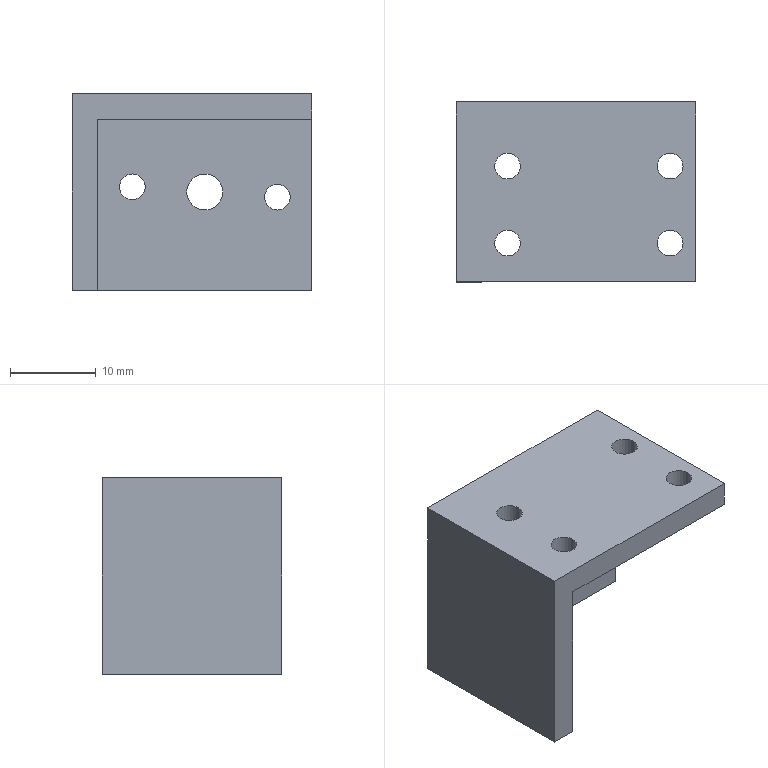Part | SolidWorks | features ICE 2, Extrusion 1 | 1 solid | 23 faces | box 28 x 21 x 23 mm | volume 4355 mm3 | cylinder 14 | plane 9 | commonest cylinder face diameters 3 x12 4.2 x2
STEP:
#1=CARTESIAN_POINT('',(8.478,12.,-10.616));
#2=VERTEX_POINT('',#1);
#3=CARTESIAN_POINT('',(8.478,12.,-7.616));
#4=VERTEX_POINT('',#3);
#5=CARTESIAN_POINT('',(8.478,12.,-9.116));
#6=DIRECTION('',(0.,1.,0.));
#7=DIRECTION('',(0.,0.,1.));
#8=AXIS2_PLACEMENT_3D('',#5,#6,#7);
#9=CIRCLE('',#8,1.5);
#10=EDGE_CURVE('',#2,#4,#9,.T.);
#11=ORIENTED_EDGE('',*,*,#10,.T.);
#12=CARTESIAN_POINT('',(8.478,9.,-7.616));
#13=VERTEX_POINT('',#12);
#14=CARTESIAN_POINT('',(8.478,12.,-7.616));
#15=DIRECTION('',(0.,-1.,0.));
#16=VECTOR('',#15,1000.);
#17=LINE('',#14,#16);
#18=EDGE_CURVE('',#4,#13,#17,.T.);
#19=ORIENTED_EDGE('',*,*,#18,.T.);
#20=CARTESIAN_POINT('',(8.478,9.,-10.616));
#21=VERTEX_POINT('',#20);
#22=CARTESIAN_POINT('',(8.478,9.,-9.116));
#23=DIRECTION('',(0.,1.,0.));
#24=DIRECTION('',(0.,0.,1.));
#25=AXIS2_PLACEMENT_3D('',#22,#23,#24);
#26=CIRCLE('',#25,1.5);
#27=EDGE_CURVE('',#21,#13,#26,.T.);
#28=ORIENTED_EDGE('',*,*,#27,.F.);
#29=CARTESIAN_POINT('',(8.478,12.,-10.616));
#30=DIRECTION('',(0.,-1.,0.));
#31=VECTOR('',#30,1000.);
#32=LINE('',#29,#31);
#33=EDGE_CURVE('',#2,#21,#32,.T.);
#34=ORIENTED_EDGE('',*,*,#33,.F.);
#35=EDGE_LOOP('',(#11,#19,#28,#34));
#36=FACE_OUTER_BOUND('',#35,.T.);
#37=CARTESIAN_POINT('',(8.478,12.,-9.116));
#38=DIRECTION('',(0.,-1.,0.));
#39=DIRECTION('',(0.,0.,-1.));
#40=AXIS2_PLACEMENT_3D('',#37,#38,#39);
#41=CYLINDRICAL_SURFACE('',#40,1.5);
#42=ADVANCED_FACE('',(#36),#41,.F.);
#43=CARTESIAN_POINT('',(-8.478,12.,-9.384));
#44=VERTEX_POINT('',#43);
#45=CARTESIAN_POINT('',(-8.478,12.,-6.384));
#46=VERTEX_POINT('',#45);
#47=CARTESIAN_POINT('',(-8.478,12.,-7.884));
#48=DIRECTION('',(0.,1.,0.));
#49=DIRECTION('',(0.,0.,1.));
#50=AXIS2_PLACEMENT_3D('',#47,#48,#49);
#51=CIRCLE('',#50,1.5);
#52=EDGE_CURVE('',#44,#46,#51,.T.);
#53=ORIENTED_EDGE('',*,*,#52,.T.);
#54=CARTESIAN_POINT('',(-8.478,9.,-6.384));
#55=VERTEX_POINT('',#54);
#56=CARTESIAN_POINT('',(-8.478,12.,-6.384));
#57=DIRECTION('',(0.,-1.,0.));
#58=VECTOR('',#57,1000.);
#59=LINE('',#56,#58);
#60=EDGE_CURVE('',#46,#55,#59,.T.);
#61=ORIENTED_EDGE('',*,*,#60,.T.);
#62=CARTESIAN_POINT('',(-8.478,9.,-9.384));
#63=VERTEX_POINT('',#62);
#64=CARTESIAN_POINT('',(-8.478,9.,-7.884));
#65=DIRECTION('',(0.,1.,0.));
#66=DIRECTION('',(0.,0.,1.));
#67=AXIS2_PLACEMENT_3D('',#64,#65,#66);
#68=CIRCLE('',#67,1.5);
#69=EDGE_CURVE('',#63,#55,#68,.T.);
#70=ORIENTED_EDGE('',*,*,#69,.F.);
#71=CARTESIAN_POINT('',(-8.478,12.,-9.384));
#72=DIRECTION('',(0.,-1.,0.));
#73=VECTOR('',#72,1000.);
#74=LINE('',#71,#73);
#75=EDGE_CURVE('',#44,#63,#74,.T.);
#76=ORIENTED_EDGE('',*,*,#75,.F.);
#77=EDGE_LOOP('',(#53,#61,#70,#76));
#78=FACE_OUTER_BOUND('',#77,.T.);
#79=CARTESIAN_POINT('',(-8.478,12.,-7.884));
#80=DIRECTION('',(0.,-1.,0.));
#81=DIRECTION('',(0.,0.,-1.));
#82=AXIS2_PLACEMENT_3D('',#79,#80,#81);
#83=CYLINDRICAL_SURFACE('',#82,1.5);
#84=ADVANCED_FACE('',(#78),#83,.F.);
#85=CARTESIAN_POINT('',(0.,12.,-10.6));
#86=VERTEX_POINT('',#85);
#87=CARTESIAN_POINT('',(0.,12.,-6.4));
#88=VERTEX_POINT('',#87);
#89=CARTESIAN_POINT('',(0.,12.,-8.5));
#90=DIRECTION('',(0.,1.,0.));
#91=DIRECTION('',(0.,0.,1.));
#92=AXIS2_PLACEMENT_3D('',#89,#90,#91);
#93=CIRCLE('',#92,2.1);
#94=EDGE_CURVE('',#86,#88,#93,.T.);
#95=ORIENTED_EDGE('',*,*,#94,.T.);
#96=CARTESIAN_POINT('',(0.,9.,-6.4));
#97=VERTEX_POINT('',#96);
#98=CARTESIAN_POINT('',(0.,12.,-6.4));
#99=DIRECTION('',(0.,-1.,0.));
#100=VECTOR('',#99,1000.);
#101=LINE('',#98,#100);
#102=EDGE_CURVE('',#88,#97,#101,.T.);
#103=ORIENTED_EDGE('',*,*,#102,.T.);
#104=CARTESIAN_POINT('',(0.,9.,-10.6));
#105=VERTEX_POINT('',#104);
#106=CARTESIAN_POINT('',(0.,9.,-8.5));
#107=DIRECTION('',(0.,1.,0.));
#108=DIRECTION('',(0.,0.,1.));
#109=AXIS2_PLACEMENT_3D('',#106,#107,#108);
#110=CIRCLE('',#109,2.1);
#111=EDGE_CURVE('',#105,#97,#110,.T.);
#112=ORIENTED_EDGE('',*,*,#111,.F.);
#113=CARTESIAN_POINT('',(0.,12.,-10.6));
#114=DIRECTION('',(0.,-1.,0.));
#115=VECTOR('',#114,1000.);
#116=LINE('',#113,#115);
#117=EDGE_CURVE('',#86,#105,#116,.T.);
#118=ORIENTED_EDGE('',*,*,#117,.F.);
#119=EDGE_LOOP('',(#95,#103,#112,#118));
#120=FACE_OUTER_BOUND('',#119,.T.);
#121=CARTESIAN_POINT('',(0.,12.,-8.5));
#122=DIRECTION('',(0.,-1.,0.));
#123=DIRECTION('',(0.,0.,-1.));
#124=AXIS2_PLACEMENT_3D('',#121,#122,#123);
#125=CYLINDRICAL_SURFACE('',#124,2.1);
#126=ADVANCED_FACE('',(#120),#125,.F.);
#127=CARTESIAN_POINT('',(-11.,-4.5,3.));
#128=VERTEX_POINT('',#127);
#129=CARTESIAN_POINT('',(-8.,-4.5,3.));
#130=VERTEX_POINT('',#129);
#131=CARTESIAN_POINT('',(-9.5,-4.5,3.));
#132=DIRECTION('',(0.,0.,1.));
#133=DIRECTION('',(1.,0.,0.));
#134=AXIS2_PLACEMENT_3D('',#131,#132,#133);
#135=CIRCLE('',#134,1.5);
#136=EDGE_CURVE('',#128,#130,#135,.T.);
#137=ORIENTED_EDGE('',*,*,#136,.T.);
#138=CARTESIAN_POINT('',(-8.,-4.5,0.));
#139=VERTEX_POINT('',#138);
#140=CARTESIAN_POINT('',(-8.,-4.5,3.));
#141=DIRECTION('',(0.,0.,-1.));
#142=VECTOR('',#141,1000.);
#143=LINE('',#140,#142);
#144=EDGE_CURVE('',#130,#139,#143,.T.);
#145=ORIENTED_EDGE('',*,*,#144,.T.);
#146=CARTESIAN_POINT('',(-11.,-4.5,0.));
#147=VERTEX_POINT('',#146);
#148=CARTESIAN_POINT('',(-9.5,-4.5,0.));
#149=DIRECTION('',(0.,0.,1.));
#150=DIRECTION('',(1.,0.,0.));
#151=AXIS2_PLACEMENT_3D('',#148,#149,#150);
#152=CIRCLE('',#151,1.5);
#153=EDGE_CURVE('',#147,#139,#152,.T.);
#154=ORIENTED_EDGE('',*,*,#153,.F.);
#155=CARTESIAN_POINT('',(-11.,-4.5,3.));
#156=DIRECTION('',(0.,0.,-1.));
#157=VECTOR('',#156,1000.);
#158=LINE('',#155,#157);
#159=EDGE_CURVE('',#128,#147,#158,.T.);
#160=ORIENTED_EDGE('',*,*,#159,.F.);
#161=EDGE_LOOP('',(#137,#145,#154,#160));
#162=FACE_OUTER_BOUND('',#161,.T.);
#163=CARTESIAN_POINT('',(-9.5,-4.5,3.));
#164=DIRECTION('',(0.,0.,-1.));
#165=DIRECTION('',(-1.,0.,0.));
#166=AXIS2_PLACEMENT_3D('',#163,#164,#165);
#167=CYLINDRICAL_SURFACE('',#166,1.5);
#168=ADVANCED_FACE('',(#162),#167,.F.);
#169=CARTESIAN_POINT('',(8.,-4.5,3.));
#170=VERTEX_POINT('',#169);
#171=CARTESIAN_POINT('',(11.,-4.5,3.));
#172=VERTEX_POINT('',#171);
#173=CARTESIAN_POINT('',(9.5,-4.5,3.));
#174=DIRECTION('',(0.,0.,1.));
#175=DIRECTION('',(1.,0.,0.));
#176=AXIS2_PLACEMENT_3D('',#173,#174,#175);
#177=CIRCLE('',#176,1.5);
#178=EDGE_CURVE('',#170,#172,#177,.T.);
#179=ORIENTED_EDGE('',*,*,#178,.T.);
#180=CARTESIAN_POINT('',(11.,-4.5,0.));
#181=VERTEX_POINT('',#180);
#182=CARTESIAN_POINT('',(11.,-4.5,3.));
#183=DIRECTION('',(0.,0.,-1.));
#184=VECTOR('',#183,1000.);
#185=LINE('',#182,#184);
#186=EDGE_CURVE('',#172,#181,#185,.T.);
#187=ORIENTED_EDGE('',*,*,#186,.T.);
#188=CARTESIAN_POINT('',(8.,-4.5,0.));
#189=VERTEX_POINT('',#188);
#190=CARTESIAN_POINT('',(9.5,-4.5,0.));
#191=DIRECTION('',(0.,0.,1.));
#192=DIRECTION('',(1.,0.,0.));
#193=AXIS2_PLACEMENT_3D('',#190,#191,#192);
#194=CIRCLE('',#193,1.5);
#195=EDGE_CURVE('',#189,#181,#194,.T.);
#196=ORIENTED_EDGE('',*,*,#195,.F.);
#197=CARTESIAN_POINT('',(8.,-4.5,3.));
#198=DIRECTION('',(0.,0.,-1.));
#199=VECTOR('',#198,1000.);
#200=LINE('',#197,#199);
#201=EDGE_CURVE('',#170,#189,#200,.T.);
#202=ORIENTED_EDGE('',*,*,#201,.F.);
#203=EDGE_LOOP('',(#179,#187,#196,#202));
#204=FACE_OUTER_BOUND('',#203,.T.);
#205=CARTESIAN_POINT('',(9.5,-4.5,3.));
#206=DIRECTION('',(0.,0.,-1.));
#207=DIRECTION('',(-1.,0.,0.));
#208=AXIS2_PLACEMENT_3D('',#205,#206,#207);
#209=CYLINDRICAL_SURFACE('',#208,1.5);
#210=ADVANCED_FACE('',(#204),#209,.F.);
#211=CARTESIAN_POINT('',(8.,4.5,3.));
#212=VERTEX_POINT('',#211);
#213=CARTESIAN_POINT('',(11.,4.5,3.));
#214=VERTEX_POINT('',#213);
#215=CARTESIAN_POINT('',(9.5,4.5,3.));
#216=DIRECTION('',(0.,0.,1.));
#217=DIRECTION('',(1.,0.,0.));
#218=AXIS2_PLACEMENT_3D('',#215,#216,#217);
#219=CIRCLE('',#218,1.5);
#220=EDGE_CURVE('',#212,#214,#219,.T.);
#221=ORIENTED_EDGE('',*,*,#220,.T.);
#222=CARTESIAN_POINT('',(11.,4.5,0.));
#223=VERTEX_POINT('',#222);
#224=CARTESIAN_POINT('',(11.,4.5,3.));
#225=DIRECTION('',(0.,0.,-1.));
#226=VECTOR('',#225,1000.);
#227=LINE('',#224,#226);
#228=EDGE_CURVE('',#214,#223,#227,.T.);
#229=ORIENTED_EDGE('',*,*,#228,.T.);
#230=CARTESIAN_POINT('',(8.,4.5,0.));
#231=VERTEX_POINT('',#230);
#232=CARTESIAN_POINT('',(9.5,4.5,0.));
#233=DIRECTION('',(0.,0.,1.));
#234=DIRECTION('',(1.,0.,0.));
#235=AXIS2_PLACEMENT_3D('',#232,#233,#234);
#236=CIRCLE('',#235,1.5);
#237=EDGE_CURVE('',#231,#223,#236,.T.);
#238=ORIENTED_EDGE('',*,*,#237,.F.);
#239=CARTESIAN_POINT('',(8.,4.5,3.));
#240=DIRECTION('',(0.,0.,-1.));
#241=VECTOR('',#240,1000.);
#242=LINE('',#239,#241);
#243=EDGE_CURVE('',#212,#231,#242,.T.);
#244=ORIENTED_EDGE('',*,*,#243,.F.);
#245=EDGE_LOOP('',(#221,#229,#238,#244));
#246=FACE_OUTER_BOUND('',#245,.T.);
#247=CARTESIAN_POINT('',(9.5,4.5,3.));
#248=DIRECTION('',(0.,0.,-1.));
#249=DIRECTION('',(-1.,0.,0.));
#250=AXIS2_PLACEMENT_3D('',#247,#248,#249);
#251=CYLINDRICAL_SURFACE('',#250,1.5);
#252=ADVANCED_FACE('',(#246),#251,.F.);
#253=CARTESIAN_POINT('',(-11.,4.5,3.));
#254=VERTEX_POINT('',#253);
#255=CARTESIAN_POINT('',(-8.,4.5,3.));
#256=VERTEX_POINT('',#255);
#257=CARTESIAN_POINT('',(-9.5,4.5,3.));
#258=DIRECTION('',(0.,0.,1.));
#259=DIRECTION('',(1.,0.,0.));
#260=AXIS2_PLACEMENT_3D('',#257,#258,#259);
#261=CIRCLE('',#260,1.5);
#262=EDGE_CURVE('',#254,#256,#261,.T.);
#263=ORIENTED_EDGE('',*,*,#262,.T.);
#264=CARTESIAN_POINT('',(-8.,4.5,0.));
#265=VERTEX_POINT('',#264);
#266=CARTESIAN_POINT('',(-8.,4.5,3.));
#267=DIRECTION('',(0.,0.,-1.));
#268=VECTOR('',#267,1000.);
#269=LINE('',#266,#268);
#270=EDGE_CURVE('',#256,#265,#269,.T.);
#271=ORIENTED_EDGE('',*,*,#270,.T.);
#272=CARTESIAN_POINT('',(-11.,4.5,0.));
#273=VERTEX_POINT('',#272);
#274=CARTESIAN_POINT('',(-9.5,4.5,0.));
#275=DIRECTION('',(0.,0.,1.));
#276=DIRECTION('',(1.,0.,0.));
#277=AXIS2_PLACEMENT_3D('',#274,#275,#276);
#278=CIRCLE('',#277,1.5);
#279=EDGE_CURVE('',#273,#265,#278,.T.);
#280=ORIENTED_EDGE('',*,*,#279,.F.);
#281=CARTESIAN_POINT('',(-11.,4.5,3.));
#282=DIRECTION('',(0.,0.,-1.));
#283=VECTOR('',#282,1000.);
#284=LINE('',#281,#283);
#285=EDGE_CURVE('',#254,#273,#284,.T.);
#286=ORIENTED_EDGE('',*,*,#285,.F.);
#287=EDGE_LOOP('',(#263,#271,#280,#286));
#288=FACE_OUTER_BOUND('',#287,.T.);
#289=CARTESIAN_POINT('',(-9.5,4.5,3.));
#290=DIRECTION('',(0.,0.,-1.));
#291=DIRECTION('',(-1.,0.,0.));
#292=AXIS2_PLACEMENT_3D('',#289,#290,#291);
#293=CYLINDRICAL_SURFACE('',#292,1.5);
#294=ADVANCED_FACE('',(#288),#293,.F.);
#295=CARTESIAN_POINT('',(12.5,-9.,3.));
#296=VERTEX_POINT('',#295);
#297=CARTESIAN_POINT('',(12.5,12.,3.));
#298=VERTEX_POINT('',#297);
#299=CARTESIAN_POINT('',(12.5,-9.,3.));
#300=DIRECTION('',(0.,1.,0.));
#301=VECTOR('',#300,1000.);
#302=LINE('',#299,#301);
#303=EDGE_CURVE('',#296,#298,#302,.T.);
#304=ORIENTED_EDGE('',*,*,#303,.T.);
#305=CARTESIAN_POINT('',(-15.5,12.,3.));
#306=VERTEX_POINT('',#305);
#307=CARTESIAN_POINT('',(-12.5,12.,3.));
#308=DIRECTION('',(1.,0.,0.));
#309=VECTOR('',#308,1000.);
#310=LINE('',#307,#309);
#311=EDGE_CURVE('',#306,#298,#310,.T.);
#312=ORIENTED_EDGE('',*,*,#311,.F.);
#313=CARTESIAN_POINT('',(-15.5,-9.,3.));
#314=VERTEX_POINT('',#313);
#315=CARTESIAN_POINT('',(-15.5,12.,3.));
#316=DIRECTION('',(0.,1.,0.));
#317=VECTOR('',#316,1000.);
#318=LINE('',#315,#317);
#319=EDGE_CURVE('',#314,#306,#318,.T.);
#320=ORIENTED_EDGE('',*,*,#319,.F.);
#321=CARTESIAN_POINT('',(-12.5,-9.,3.));
#322=DIRECTION('',(1.,0.,0.));
#323=VECTOR('',#322,1000.);
#324=LINE('',#321,#323);
#325=EDGE_CURVE('',#314,#296,#324,.T.);
#326=ORIENTED_EDGE('',*,*,#325,.T.);
#327=EDGE_LOOP('',(#304,#312,#320,#326));
#328=FACE_OUTER_BOUND('',#327,.T.);
#329=ORIENTED_EDGE('',*,*,#262,.F.);
#330=CARTESIAN_POINT('',(-9.5,4.5,3.));
#331=DIRECTION('',(0.,0.,1.));
#332=DIRECTION('',(1.,0.,0.));
#333=AXIS2_PLACEMENT_3D('',#330,#331,#332);
#334=CIRCLE('',#333,1.5);
#335=EDGE_CURVE('',#256,#254,#334,.T.);
#336=ORIENTED_EDGE('',*,*,#335,.F.);
#337=EDGE_LOOP('',(#329,#336));
#338=FACE_BOUND('',#337,.T.);
#339=ORIENTED_EDGE('',*,*,#220,.F.);
#340=CARTESIAN_POINT('',(9.5,4.5,3.));
#341=DIRECTION('',(0.,0.,1.));
#342=DIRECTION('',(1.,0.,0.));
#343=AXIS2_PLACEMENT_3D('',#340,#341,#342);
#344=CIRCLE('',#343,1.5);
#345=EDGE_CURVE('',#214,#212,#344,.T.);
#346=ORIENTED_EDGE('',*,*,#345,.F.);
#347=EDGE_LOOP('',(#339,#346));
#348=FACE_BOUND('',#347,.T.);
#349=ORIENTED_EDGE('',*,*,#178,.F.);
#350=CARTESIAN_POINT('',(9.5,-4.5,3.));
#351=DIRECTION('',(0.,0.,1.));
#352=DIRECTION('',(1.,0.,0.));
#353=AXIS2_PLACEMENT_3D('',#350,#351,#352);
#354=CIRCLE('',#353,1.5);
#355=EDGE_CURVE('',#172,#170,#354,.T.);
#356=ORIENTED_EDGE('',*,*,#355,.F.);
#357=EDGE_LOOP('',(#349,#356));
#358=FACE_BOUND('',#357,.T.);
#359=ORIENTED_EDGE('',*,*,#136,.F.);
#360=CARTESIAN_POINT('',(-9.5,-4.5,3.));
#361=DIRECTION('',(0.,0.,1.));
#362=DIRECTION('',(1.,0.,0.));
#363=AXIS2_PLACEMENT_3D('',#360,#361,#362);
#364=CIRCLE('',#363,1.5);
#365=EDGE_CURVE('',#130,#128,#364,.T.);
#366=ORIENTED_EDGE('',*,*,#365,.F.);
#367=EDGE_LOOP('',(#359,#366));
#368=FACE_BOUND('',#367,.T.);
#369=CARTESIAN_POINT('',(0.,0.,3.));
#370=DIRECTION('',(0.,0.,-1.));
#371=DIRECTION('',(-1.,0.,0.));
#372=AXIS2_PLACEMENT_3D('',#369,#370,#371);
#373=PLANE('',#372);
#374=ADVANCED_FACE('',(#328,#338,#348,#358,#368),#373,.F.);
#375=ORIENTED_EDGE('',*,*,#195,.T.);
#376=CARTESIAN_POINT('',(9.5,-4.5,0.));
#377=DIRECTION('',(0.,0.,1.));
#378=DIRECTION('',(1.,0.,0.));
#379=AXIS2_PLACEMENT_3D('',#376,#377,#378);
#380=CIRCLE('',#379,1.5);
#381=EDGE_CURVE('',#181,#189,#380,.T.);
#382=ORIENTED_EDGE('',*,*,#381,.T.);
#383=EDGE_LOOP('',(#375,#382));
#384=FACE_BOUND('',#383,.T.);
#385=ORIENTED_EDGE('',*,*,#279,.T.);
#386=CARTESIAN_POINT('',(-9.5,4.5,0.));
#387=DIRECTION('',(0.,0.,1.));
#388=DIRECTION('',(1.,0.,0.));
#389=AXIS2_PLACEMENT_3D('',#386,#387,#388);
#390=CIRCLE('',#389,1.5);
#391=EDGE_CURVE('',#265,#273,#390,.T.);
#392=ORIENTED_EDGE('',*,*,#391,.T.);
#393=EDGE_LOOP('',(#385,#392));
#394=FACE_BOUND('',#393,.T.);
#395=CARTESIAN_POINT('',(12.5,-9.,0.));
#396=VERTEX_POINT('',#395);
#397=CARTESIAN_POINT('',(12.5,9.,0.));
#398=VERTEX_POINT('',#397);
#399=CARTESIAN_POINT('',(12.5,-9.,0.));
#400=DIRECTION('',(0.,1.,0.));
#401=VECTOR('',#400,1000.);
#402=LINE('',#399,#401);
#403=EDGE_CURVE('',#396,#398,#402,.T.);
#404=ORIENTED_EDGE('',*,*,#403,.F.);
#405=CARTESIAN_POINT('',(-12.5,-9.,0.));
#406=VERTEX_POINT('',#405);
#407=CARTESIAN_POINT('',(-12.5,-9.,0.));
#408=DIRECTION('',(1.,0.,0.));
#409=VECTOR('',#408,1000.);
#410=LINE('',#407,#409);
#411=EDGE_CURVE('',#406,#396,#410,.T.);
#412=ORIENTED_EDGE('',*,*,#411,.F.);
#413=CARTESIAN_POINT('',(-12.5,9.,0.));
#414=VERTEX_POINT('',#413);
#415=CARTESIAN_POINT('',(-12.5,-9.,0.));
#416=DIRECTION('',(0.,-1.,0.));
#417=VECTOR('',#416,1000.);
#418=LINE('',#415,#417);
#419=EDGE_CURVE('',#414,#406,#418,.T.);
#420=ORIENTED_EDGE('',*,*,#419,.F.);
#421=CARTESIAN_POINT('',(-12.5,9.,0.));
#422=DIRECTION('',(-1.,0.,0.));
#423=VECTOR('',#422,1000.);
#424=LINE('',#421,#423);
#425=EDGE_CURVE('',#398,#414,#424,.T.);
#426=ORIENTED_EDGE('',*,*,#425,.F.);
#427=EDGE_LOOP('',(#404,#412,#420,#426));
#428=FACE_OUTER_BOUND('',#427,.T.);
#429=ORIENTED_EDGE('',*,*,#237,.T.);
#430=CARTESIAN_POINT('',(9.5,4.5,0.));
#431=DIRECTION('',(0.,0.,1.));
#432=DIRECTION('',(1.,0.,0.));
#433=AXIS2_PLACEMENT_3D('',#430,#431,#432);
#434=CIRCLE('',#433,1.5);
#435=EDGE_CURVE('',#223,#231,#434,.T.);
#436=ORIENTED_EDGE('',*,*,#435,.T.);
#437=EDGE_LOOP('',(#429,#436));
#438=FACE_BOUND('',#437,.T.);
#439=ORIENTED_EDGE('',*,*,#153,.T.);
#440=CARTESIAN_POINT('',(-9.5,-4.5,0.));
#441=DIRECTION('',(0.,0.,1.));
#442=DIRECTION('',(1.,0.,0.));
#443=AXIS2_PLACEMENT_3D('',#440,#441,#442);
#444=CIRCLE('',#443,1.5);
#445=EDGE_CURVE('',#139,#147,#444,.T.);
#446=ORIENTED_EDGE('',*,*,#445,.T.);
#447=EDGE_LOOP('',(#439,#446));
#448=FACE_BOUND('',#447,.T.);
#449=CARTESIAN_POINT('',(0.,0.,0.));
#450=DIRECTION('',(0.,0.,-1.));
#451=DIRECTION('',(-1.,0.,0.));
#452=AXIS2_PLACEMENT_3D('',#449,#450,#451);
#453=PLANE('',#452);
#454=ADVANCED_FACE('',(#384,#394,#428,#438,#448),#453,.T.);
#455=ORIENTED_EDGE('',*,*,#403,.T.);
#456=CARTESIAN_POINT('',(12.5,9.,-20.));
#457=VERTEX_POINT('',#456);
#458=CARTESIAN_POINT('',(12.5,9.,3.));
#459=DIRECTION('',(0.,0.,-1.));
#460=VECTOR('',#459,1000.);
#461=LINE('',#458,#460);
#462=EDGE_CURVE('',#398,#457,#461,.T.);
#463=ORIENTED_EDGE('',*,*,#462,.T.);
#464=CARTESIAN_POINT('',(12.5,12.,-20.));
#465=VERTEX_POINT('',#464);
#466=CARTESIAN_POINT('',(12.5,12.,-20.));
#467=DIRECTION('',(0.,-1.,0.));
#468=VECTOR('',#467,1000.);
#469=LINE('',#466,#468);
#470=EDGE_CURVE('',#465,#457,#469,.T.);
#471=ORIENTED_EDGE('',*,*,#470,.F.);
#472=CARTESIAN_POINT('',(12.5,12.,3.));
#473=DIRECTION('',(0.,0.,-1.));
#474=VECTOR('',#473,1000.);
#475=LINE('',#472,#474);
#476=EDGE_CURVE('',#298,#465,#475,.T.);
#477=ORIENTED_EDGE('',*,*,#476,.F.);
#478=ORIENTED_EDGE('',*,*,#303,.F.);
#479=CARTESIAN_POINT('',(12.5,-9.,3.));
#480=DIRECTION('',(0.,0.,-1.));
#481=VECTOR('',#480,1000.);
#482=LINE('',#479,#481);
#483=EDGE_CURVE('',#296,#396,#482,.T.);
#484=ORIENTED_EDGE('',*,*,#483,.T.);
#485=EDGE_LOOP('',(#455,#463,#471,#477,#478,#484));
#486=FACE_OUTER_BOUND('',#485,.T.);
#487=CARTESIAN_POINT('',(12.5,-9.,3.));
#488=DIRECTION('',(-1.,0.,0.));
#489=DIRECTION('',(0.,0.,1.));
#490=AXIS2_PLACEMENT_3D('',#487,#488,#489);
#491=PLANE('',#490);
#492=ADVANCED_FACE('',(#486),#491,.F.);
#493=ORIENTED_EDGE('',*,*,#411,.T.);
#494=ORIENTED_EDGE('',*,*,#483,.F.);
#495=ORIENTED_EDGE('',*,*,#325,.F.);
#496=CARTESIAN_POINT('',(-15.5,-9.,-20.));
#497=VERTEX_POINT('',#496);
#498=CARTESIAN_POINT('',(-15.5,-9.,3.));
#499=DIRECTION('',(0.,0.,1.));
#500=VECTOR('',#499,1000.);
#501=LINE('',#498,#500);
#502=EDGE_CURVE('',#497,#314,#501,.T.);
#503=ORIENTED_EDGE('',*,*,#502,.F.);
#504=CARTESIAN_POINT('',(-12.5,-9.,-20.));
#505=VERTEX_POINT('',#504);
#506=CARTESIAN_POINT('',(-15.5,-9.,-20.));
#507=DIRECTION('',(1.,0.,0.));
#508=VECTOR('',#507,1000.);
#509=LINE('',#506,#508);
#510=EDGE_CURVE('',#497,#505,#509,.T.);
#511=ORIENTED_EDGE('',*,*,#510,.T.);
#512=CARTESIAN_POINT('',(-12.5,-9.,3.));
#513=DIRECTION('',(0.,0.,1.));
#514=VECTOR('',#513,1000.);
#515=LINE('',#512,#514);
#516=EDGE_CURVE('',#505,#406,#515,.T.);
#517=ORIENTED_EDGE('',*,*,#516,.T.);
#518=EDGE_LOOP('',(#493,#494,#495,#503,#511,#517));
#519=FACE_OUTER_BOUND('',#518,.T.);
#520=CARTESIAN_POINT('',(-12.5,-9.,3.));
#521=DIRECTION('',(0.,1.,0.));
#522=DIRECTION('',(0.,0.,1.));
#523=AXIS2_PLACEMENT_3D('',#520,#521,#522);
#524=PLANE('',#523);
#525=ADVANCED_FACE('',(#519),#524,.F.);
#526=ORIENTED_EDGE('',*,*,#270,.F.);
#527=ORIENTED_EDGE('',*,*,#335,.T.);
#528=ORIENTED_EDGE('',*,*,#285,.T.);
#529=ORIENTED_EDGE('',*,*,#391,.F.);
#530=EDGE_LOOP('',(#526,#527,#528,#529));
#531=FACE_OUTER_BOUND('',#530,.T.);
#532=CARTESIAN_POINT('',(-9.5,4.5,3.));
#533=DIRECTION('',(0.,0.,-1.));
#534=DIRECTION('',(-1.,0.,0.));
#535=AXIS2_PLACEMENT_3D('',#532,#533,#534);
#536=CYLINDRICAL_SURFACE('',#535,1.5);
#537=ADVANCED_FACE('',(#531),#536,.F.);
#538=ORIENTED_EDGE('',*,*,#228,.F.);
#539=ORIENTED_EDGE('',*,*,#345,.T.);
#540=ORIENTED_EDGE('',*,*,#243,.T.);
#541=ORIENTED_EDGE('',*,*,#435,.F.);
#542=EDGE_LOOP('',(#538,#539,#540,#541));
#543=FACE_OUTER_BOUND('',#542,.T.);
#544=CARTESIAN_POINT('',(9.5,4.5,3.));
#545=DIRECTION('',(0.,0.,-1.));
#546=DIRECTION('',(-1.,0.,0.));
#547=AXIS2_PLACEMENT_3D('',#544,#545,#546);
#548=CYLINDRICAL_SURFACE('',#547,1.5);
#549=ADVANCED_FACE('',(#543),#548,.F.);
#550=ORIENTED_EDGE('',*,*,#186,.F.);
#551=ORIENTED_EDGE('',*,*,#355,.T.);
#552=ORIENTED_EDGE('',*,*,#201,.T.);
#553=ORIENTED_EDGE('',*,*,#381,.F.);
#554=EDGE_LOOP('',(#550,#551,#552,#553));
#555=FACE_OUTER_BOUND('',#554,.T.);
#556=CARTESIAN_POINT('',(9.5,-4.5,3.));
#557=DIRECTION('',(0.,0.,-1.));
#558=DIRECTION('',(-1.,0.,0.));
#559=AXIS2_PLACEMENT_3D('',#556,#557,#558);
#560=CYLINDRICAL_SURFACE('',#559,1.5);
#561=ADVANCED_FACE('',(#555),#560,.F.);
#562=ORIENTED_EDGE('',*,*,#144,.F.);
#563=ORIENTED_EDGE('',*,*,#365,.T.);
#564=ORIENTED_EDGE('',*,*,#159,.T.);
#565=ORIENTED_EDGE('',*,*,#445,.F.);
#566=EDGE_LOOP('',(#562,#563,#564,#565));
#567=FACE_OUTER_BOUND('',#566,.T.);
#568=CARTESIAN_POINT('',(-9.5,-4.5,3.));
#569=DIRECTION('',(0.,0.,-1.));
#570=DIRECTION('',(-1.,0.,0.));
#571=AXIS2_PLACEMENT_3D('',#568,#569,#570);
#572=CYLINDRICAL_SURFACE('',#571,1.5);
#573=ADVANCED_FACE('',(#567),#572,.F.);
#574=CARTESIAN_POINT('',(-15.5,12.,-20.));
#575=VERTEX_POINT('',#574);
#576=CARTESIAN_POINT('',(-12.5,12.,-20.));
#577=DIRECTION('',(-1.,0.,0.));
#578=VECTOR('',#577,1000.);
#579=LINE('',#576,#578);
#580=EDGE_CURVE('',#465,#575,#579,.T.);
#581=ORIENTED_EDGE('',*,*,#580,.T.);
#582=CARTESIAN_POINT('',(-15.5,12.,3.));
#583=DIRECTION('',(0.,0.,-1.));
#584=VECTOR('',#583,1000.);
#585=LINE('',#582,#584);
#586=EDGE_CURVE('',#306,#575,#585,.T.);
#587=ORIENTED_EDGE('',*,*,#586,.F.);
#588=ORIENTED_EDGE('',*,*,#311,.T.);
#589=ORIENTED_EDGE('',*,*,#476,.T.);
#590=EDGE_LOOP('',(#581,#587,#588,#589));
#591=FACE_OUTER_BOUND('',#590,.T.);
#592=ORIENTED_EDGE('',*,*,#94,.F.);
#593=CARTESIAN_POINT('',(0.,12.,-8.5));
#594=DIRECTION('',(0.,1.,0.));
#595=DIRECTION('',(0.,0.,1.));
#596=AXIS2_PLACEMENT_3D('',#593,#594,#595);
#597=CIRCLE('',#596,2.1);
#598=EDGE_CURVE('',#88,#86,#597,.T.);
#599=ORIENTED_EDGE('',*,*,#598,.F.);
#600=EDGE_LOOP('',(#592,#599));
#601=FACE_BOUND('',#600,.T.);
#602=ORIENTED_EDGE('',*,*,#52,.F.);
#603=CARTESIAN_POINT('',(-8.478,12.,-7.884));
#604=DIRECTION('',(0.,1.,0.));
#605=DIRECTION('',(0.,0.,1.));
#606=AXIS2_PLACEMENT_3D('',#603,#604,#605);
#607=CIRCLE('',#606,1.5);
#608=EDGE_CURVE('',#46,#44,#607,.T.);
#609=ORIENTED_EDGE('',*,*,#608,.F.);
#610=EDGE_LOOP('',(#602,#609));
#611=FACE_BOUND('',#610,.T.);
#612=ORIENTED_EDGE('',*,*,#10,.F.);
#613=CARTESIAN_POINT('',(8.478,12.,-9.116));
#614=DIRECTION('',(0.,1.,0.));
#615=DIRECTION('',(0.,0.,1.));
#616=AXIS2_PLACEMENT_3D('',#613,#614,#615);
#617=CIRCLE('',#616,1.5);
#618=EDGE_CURVE('',#4,#2,#617,.T.);
#619=ORIENTED_EDGE('',*,*,#618,.F.);
#620=EDGE_LOOP('',(#612,#619));
#621=FACE_BOUND('',#620,.T.);
#622=CARTESIAN_POINT('',(0.,12.,0.));
#623=DIRECTION('',(0.,-1.,0.));
#624=DIRECTION('',(0.,0.,-1.));
#625=AXIS2_PLACEMENT_3D('',#622,#623,#624);
#626=PLANE('',#625);
#627=ADVANCED_FACE('',(#591,#601,#611,#621),#626,.F.);
#628=ORIENTED_EDGE('',*,*,#69,.T.);
#629=CARTESIAN_POINT('',(-8.478,9.,-7.884));
#630=DIRECTION('',(0.,1.,0.));
#631=DIRECTION('',(0.,0.,1.));
#632=AXIS2_PLACEMENT_3D('',#629,#630,#631);
#633=CIRCLE('',#632,1.5);
#634=EDGE_CURVE('',#55,#63,#633,.T.);
#635=ORIENTED_EDGE('',*,*,#634,.T.);
#636=EDGE_LOOP('',(#628,#635));
#637=FACE_BOUND('',#636,.T.);
#638=ORIENTED_EDGE('',*,*,#462,.F.);
#639=ORIENTED_EDGE('',*,*,#425,.T.);
#640=CARTESIAN_POINT('',(-12.5,9.,-20.));
#641=VERTEX_POINT('',#640);
#642=CARTESIAN_POINT('',(-12.5,9.,3.));
#643=DIRECTION('',(0.,0.,1.));
#644=VECTOR('',#643,1000.);
#645=LINE('',#642,#644);
#646=EDGE_CURVE('',#641,#414,#645,.T.);
#647=ORIENTED_EDGE('',*,*,#646,.F.);
#648=CARTESIAN_POINT('',(-12.5,9.,-20.));
#649=DIRECTION('',(-1.,0.,0.));
#650=VECTOR('',#649,1000.);
#651=LINE('',#648,#650);
#652=EDGE_CURVE('',#457,#641,#651,.T.);
#653=ORIENTED_EDGE('',*,*,#652,.F.);
#654=EDGE_LOOP('',(#638,#639,#647,#653));
#655=FACE_OUTER_BOUND('',#654,.T.);
#656=ORIENTED_EDGE('',*,*,#111,.T.);
#657=CARTESIAN_POINT('',(0.,9.,-8.5));
#658=DIRECTION('',(0.,1.,0.));
#659=DIRECTION('',(0.,0.,1.));
#660=AXIS2_PLACEMENT_3D('',#657,#658,#659);
#661=CIRCLE('',#660,2.1);
#662=EDGE_CURVE('',#97,#105,#661,.T.);
#663=ORIENTED_EDGE('',*,*,#662,.T.);
#664=EDGE_LOOP('',(#656,#663));
#665=FACE_BOUND('',#664,.T.);
#666=ORIENTED_EDGE('',*,*,#27,.T.);
#667=CARTESIAN_POINT('',(8.478,9.,-9.116));
#668=DIRECTION('',(0.,1.,0.));
#669=DIRECTION('',(0.,0.,1.));
#670=AXIS2_PLACEMENT_3D('',#667,#668,#669);
#671=CIRCLE('',#670,1.5);
#672=EDGE_CURVE('',#13,#21,#671,.T.);
#673=ORIENTED_EDGE('',*,*,#672,.T.);
#674=EDGE_LOOP('',(#666,#673));
#675=FACE_BOUND('',#674,.T.);
#676=CARTESIAN_POINT('',(0.,9.,0.));
#677=DIRECTION('',(0.,-1.,0.));
#678=DIRECTION('',(0.,0.,-1.));
#679=AXIS2_PLACEMENT_3D('',#676,#677,#678);
#680=PLANE('',#679);
#681=ADVANCED_FACE('',(#637,#655,#665,#675),#680,.T.);
#682=ORIENTED_EDGE('',*,*,#652,.T.);
#683=CARTESIAN_POINT('',(-12.5,12.,-20.));
#684=DIRECTION('',(0.,-1.,0.));
#685=VECTOR('',#684,1000.);
#686=LINE('',#683,#685);
#687=EDGE_CURVE('',#641,#505,#686,.T.);
#688=ORIENTED_EDGE('',*,*,#687,.T.);
#689=ORIENTED_EDGE('',*,*,#510,.F.);
#690=CARTESIAN_POINT('',(-15.5,12.,-20.));
#691=DIRECTION('',(0.,-1.,0.));
#692=VECTOR('',#691,1000.);
#693=LINE('',#690,#692);
#694=EDGE_CURVE('',#575,#497,#693,.T.);
#695=ORIENTED_EDGE('',*,*,#694,.F.);
#696=ORIENTED_EDGE('',*,*,#580,.F.);
#697=ORIENTED_EDGE('',*,*,#470,.T.);
#698=EDGE_LOOP('',(#682,#688,#689,#695,#696,#697));
#699=FACE_OUTER_BOUND('',#698,.T.);
#700=CARTESIAN_POINT('',(-12.5,12.,-20.));
#701=DIRECTION('',(0.,0.,1.));
#702=DIRECTION('',(1.,0.,0.));
#703=AXIS2_PLACEMENT_3D('',#700,#701,#702);
#704=PLANE('',#703);
#705=ADVANCED_FACE('',(#699),#704,.F.);
#706=ORIENTED_EDGE('',*,*,#102,.F.);
#707=ORIENTED_EDGE('',*,*,#598,.T.);
#708=ORIENTED_EDGE('',*,*,#117,.T.);
#709=ORIENTED_EDGE('',*,*,#662,.F.);
#710=EDGE_LOOP('',(#706,#707,#708,#709));
#711=FACE_OUTER_BOUND('',#710,.T.);
#712=CARTESIAN_POINT('',(0.,12.,-8.5));
#713=DIRECTION('',(0.,-1.,0.));
#714=DIRECTION('',(0.,0.,-1.));
#715=AXIS2_PLACEMENT_3D('',#712,#713,#714);
#716=CYLINDRICAL_SURFACE('',#715,2.1);
#717=ADVANCED_FACE('',(#711),#716,.F.);
#718=ORIENTED_EDGE('',*,*,#60,.F.);
#719=ORIENTED_EDGE('',*,*,#608,.T.);
#720=ORIENTED_EDGE('',*,*,#75,.T.);
#721=ORIENTED_EDGE('',*,*,#634,.F.);
#722=EDGE_LOOP('',(#718,#719,#720,#721));
#723=FACE_OUTER_BOUND('',#722,.T.);
#724=CARTESIAN_POINT('',(-8.478,12.,-7.884));
#725=DIRECTION('',(0.,-1.,0.));
#726=DIRECTION('',(0.,0.,-1.));
#727=AXIS2_PLACEMENT_3D('',#724,#725,#726);
#728=CYLINDRICAL_SURFACE('',#727,1.5);
#729=ADVANCED_FACE('',(#723),#728,.F.);
#730=ORIENTED_EDGE('',*,*,#18,.F.);
#731=ORIENTED_EDGE('',*,*,#618,.T.);
#732=ORIENTED_EDGE('',*,*,#33,.T.);
#733=ORIENTED_EDGE('',*,*,#672,.F.);
#734=EDGE_LOOP('',(#730,#731,#732,#733));
#735=FACE_OUTER_BOUND('',#734,.T.);
#736=CARTESIAN_POINT('',(8.478,12.,-9.116));
#737=DIRECTION('',(0.,-1.,0.));
#738=DIRECTION('',(0.,0.,-1.));
#739=AXIS2_PLACEMENT_3D('',#736,#737,#738);
#740=CYLINDRICAL_SURFACE('',#739,1.5);
#741=ADVANCED_FACE('',(#735),#740,.F.);
#742=ORIENTED_EDGE('',*,*,#319,.T.);
#743=ORIENTED_EDGE('',*,*,#586,.T.);
#744=ORIENTED_EDGE('',*,*,#694,.T.);
#745=ORIENTED_EDGE('',*,*,#502,.T.);
#746=EDGE_LOOP('',(#742,#743,#744,#745));
#747=FACE_OUTER_BOUND('',#746,.T.);
#748=CARTESIAN_POINT('',(-15.5,0.,0.));
#749=DIRECTION('',(1.,0.,0.));
#750=DIRECTION('',(0.,0.,-1.));
#751=AXIS2_PLACEMENT_3D('',#748,#749,#750);
#752=PLANE('',#751);
#753=ADVANCED_FACE('',(#747),#752,.F.);
#754=ORIENTED_EDGE('',*,*,#646,.T.);
#755=ORIENTED_EDGE('',*,*,#419,.T.);
#756=ORIENTED_EDGE('',*,*,#516,.F.);
#757=ORIENTED_EDGE('',*,*,#687,.F.);
#758=EDGE_LOOP('',(#754,#755,#756,#757));
#759=FACE_OUTER_BOUND('',#758,.T.);
#760=CARTESIAN_POINT('',(-12.5,0.,0.));
#761=DIRECTION('',(1.,0.,0.));
#762=DIRECTION('',(0.,0.,-1.));
#763=AXIS2_PLACEMENT_3D('',#760,#761,#762);
#764=PLANE('',#763);
#765=ADVANCED_FACE('',(#759),#764,.T.);
#766=CLOSED_SHELL('',(#42,#84,#126,#168,#210,#252,#294,#374,#454,#492,#525,#537,#549,#561,#573,#627,#681,#705,#717,#729,#741,#753,#765));
#767=MANIFOLD_SOLID_BREP('',#766);
#768=CARTESIAN_POINT('',(0.,0.,0.));
#769=DIRECTION('',(0.,0.,1.));
#770=DIRECTION('',(1.,0.,0.));
#771=AXIS2_PLACEMENT_3D('',#768,#769,#770);
#772=(LENGTH_UNIT()NAMED_UNIT(*)SI_UNIT(.MILLI.,.METRE.));
#773=UNCERTAINTY_MEASURE_WITH_UNIT(LENGTH_MEASURE(0.00001),#772,'','');
#774=(NAMED_UNIT(*)PLANE_ANGLE_UNIT()SI_UNIT($,.RADIAN.));
#775=(NAMED_UNIT(*)SI_UNIT($,.STERADIAN.)SOLID_ANGLE_UNIT());
#776=(GEOMETRIC_REPRESENTATION_CONTEXT(3)GLOBAL_UNCERTAINTY_ASSIGNED_CONTEXT((#773))GLOBAL_UNIT_ASSIGNED_CONTEXT((#772,#774,#775))REPRESENTATION_CONTEXT('',''));
#777=ADVANCED_BREP_SHAPE_REPRESENTATION('',(#767,#771),#776);